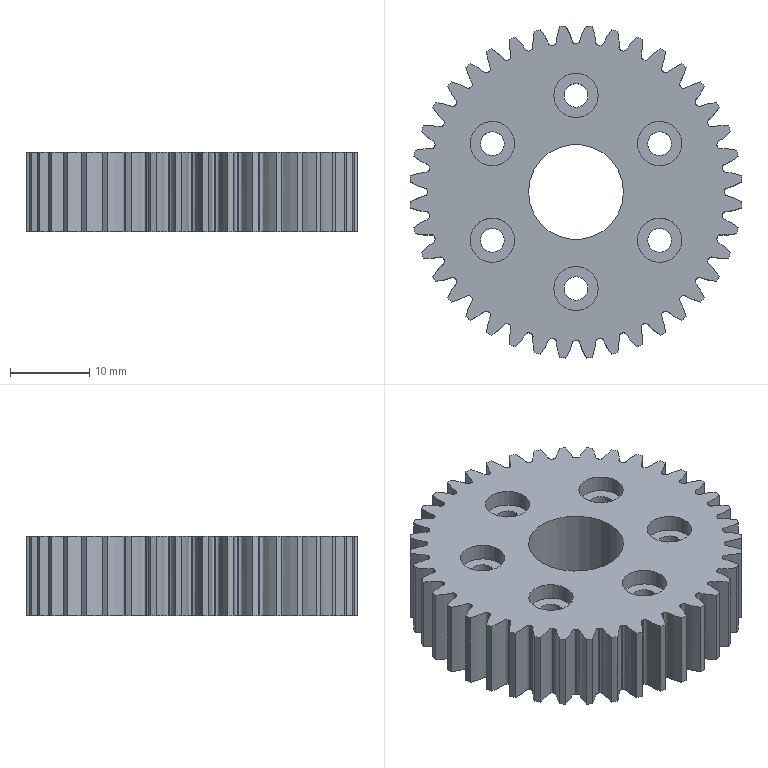Part | SolidWorks | features ICE 4, CirPattern 1, Extrusion 1, RefAxis 1 | 1 solid | 195 faces | box 41.923 x 41.923 x 10 mm | volume 10682 mm3 | cylinder 107 | spline 80 | plane 8 | commonest cylinder face diameters 37.5 x41 42 x40 3 x12 5.6 x12 12 x2